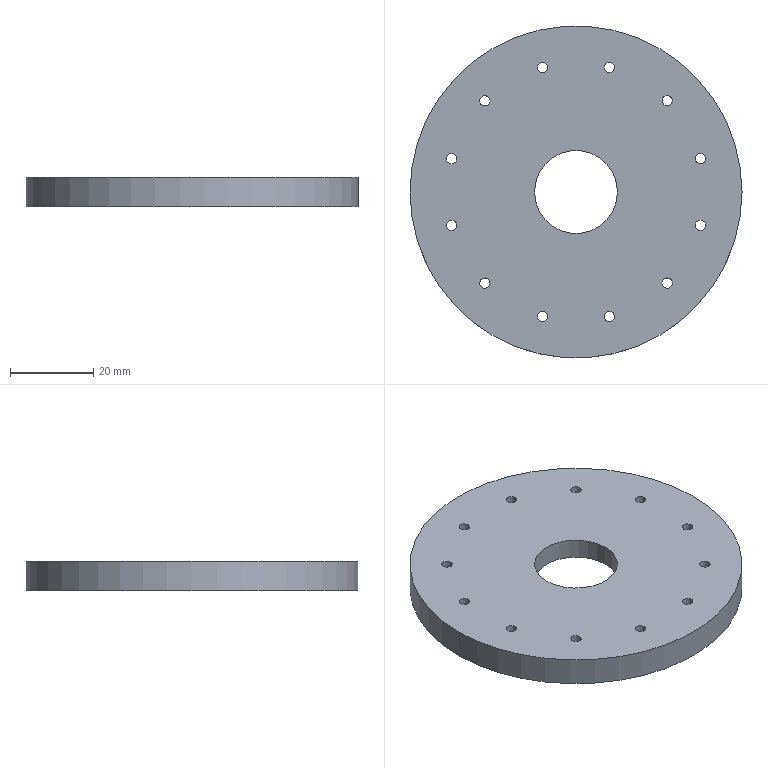Part | NX | features DATUM_CSYS 7, EXTRUDE 7, SKETCH 6, REPLACE_FACE 1 | 1 solid | 18 faces | box 80 x 80 x 7 mm | volume 31789 mm3 | cylinder 15 | plane 3 | commonest cylinder face diameters 2.5 x12 20 x1 30 x1 80 x1
STEP:
#1=CARTESIAN_POINT('',(10.,0.,7.));
#2=VERTEX_POINT('',#1);
#3=CARTESIAN_POINT('',(0.,0.,7.));
#4=DIRECTION('',(0.,0.,1.));
#5=DIRECTION('',(1.,0.,0.));
#6=AXIS2_PLACEMENT_3D('',#3,#4,#5);
#7=CIRCLE('',#6,10.);
#8=EDGE_CURVE('',#2,#2,#7,.T.);
#9=ORIENTED_EDGE('',*,*,#8,.F.);
#10=EDGE_LOOP('',(#9));
#11=FACE_BOUND('',#10,.T.);
#12=CARTESIAN_POINT('',(-28.761,-8.042,7.));
#13=VERTEX_POINT('',#12);
#14=CARTESIAN_POINT('',(-30.011,-8.042,7.));
#15=DIRECTION('',(0.,0.,1.));
#16=DIRECTION('',(1.,0.,0.));
#17=AXIS2_PLACEMENT_3D('',#14,#15,#16);
#18=CIRCLE('',#17,1.25);
#19=EDGE_CURVE('',#13,#13,#18,.T.);
#20=ORIENTED_EDGE('',*,*,#19,.F.);
#21=EDGE_LOOP('',(#20));
#22=FACE_BOUND('',#21,.T.);
#23=CARTESIAN_POINT('',(40.,0.,7.));
#24=VERTEX_POINT('',#23);
#25=CARTESIAN_POINT('',(0.,0.,7.));
#26=DIRECTION('',(0.,0.,1.));
#27=DIRECTION('',(1.,0.,0.));
#28=AXIS2_PLACEMENT_3D('',#25,#26,#27);
#29=CIRCLE('',#28,40.);
#30=EDGE_CURVE('',#24,#24,#29,.T.);
#31=ORIENTED_EDGE('',*,*,#30,.T.);
#32=EDGE_LOOP('',(#31));
#33=FACE_BOUND('',#32,.T.);
#34=CARTESIAN_POINT('',(31.261,8.042,7.));
#35=VERTEX_POINT('',#34);
#36=CARTESIAN_POINT('',(30.011,8.042,7.));
#37=DIRECTION('',(0.,0.,1.));
#38=DIRECTION('',(1.,0.,0.));
#39=AXIS2_PLACEMENT_3D('',#36,#37,#38);
#40=CIRCLE('',#39,1.25);
#41=EDGE_CURVE('',#35,#35,#40,.T.);
#42=ORIENTED_EDGE('',*,*,#41,.F.);
#43=EDGE_LOOP('',(#42));
#44=FACE_BOUND('',#43,.T.);
#45=CARTESIAN_POINT('',(31.261,-8.042,7.));
#46=VERTEX_POINT('',#45);
#47=CARTESIAN_POINT('',(30.011,-8.042,7.));
#48=DIRECTION('',(0.,0.,1.));
#49=DIRECTION('',(1.,0.,0.));
#50=AXIS2_PLACEMENT_3D('',#47,#48,#49);
#51=CIRCLE('',#50,1.25);
#52=EDGE_CURVE('',#46,#46,#51,.T.);
#53=ORIENTED_EDGE('',*,*,#52,.F.);
#54=EDGE_LOOP('',(#53));
#55=FACE_BOUND('',#54,.T.);
#56=CARTESIAN_POINT('',(23.22,21.97,7.));
#57=VERTEX_POINT('',#56);
#58=CARTESIAN_POINT('',(21.97,21.97,7.));
#59=DIRECTION('',(0.,0.,1.));
#60=DIRECTION('',(1.,0.,0.));
#61=AXIS2_PLACEMENT_3D('',#58,#59,#60);
#62=CIRCLE('',#61,1.25);
#63=EDGE_CURVE('',#57,#57,#62,.T.);
#64=ORIENTED_EDGE('',*,*,#63,.F.);
#65=EDGE_LOOP('',(#64));
#66=FACE_BOUND('',#65,.T.);
#67=CARTESIAN_POINT('',(9.292,30.011,7.));
#68=VERTEX_POINT('',#67);
#69=CARTESIAN_POINT('',(8.042,30.011,7.));
#70=DIRECTION('',(0.,0.,1.));
#71=DIRECTION('',(1.,0.,0.));
#72=AXIS2_PLACEMENT_3D('',#69,#70,#71);
#73=CIRCLE('',#72,1.25);
#74=EDGE_CURVE('',#68,#68,#73,.T.);
#75=ORIENTED_EDGE('',*,*,#74,.F.);
#76=EDGE_LOOP('',(#75));
#77=FACE_BOUND('',#76,.T.);
#78=CARTESIAN_POINT('',(23.22,-21.97,7.));
#79=VERTEX_POINT('',#78);
#80=CARTESIAN_POINT('',(21.97,-21.97,7.));
#81=DIRECTION('',(0.,0.,1.));
#82=DIRECTION('',(1.,0.,0.));
#83=AXIS2_PLACEMENT_3D('',#80,#81,#82);
#84=CIRCLE('',#83,1.25);
#85=EDGE_CURVE('',#79,#79,#84,.T.);
#86=ORIENTED_EDGE('',*,*,#85,.F.);
#87=EDGE_LOOP('',(#86));
#88=FACE_BOUND('',#87,.T.);
#89=CARTESIAN_POINT('',(9.292,-30.011,7.));
#90=VERTEX_POINT('',#89);
#91=CARTESIAN_POINT('',(8.042,-30.011,7.));
#92=DIRECTION('',(0.,0.,1.));
#93=DIRECTION('',(1.,0.,0.));
#94=AXIS2_PLACEMENT_3D('',#91,#92,#93);
#95=CIRCLE('',#94,1.25);
#96=EDGE_CURVE('',#90,#90,#95,.T.);
#97=ORIENTED_EDGE('',*,*,#96,.F.);
#98=EDGE_LOOP('',(#97));
#99=FACE_BOUND('',#98,.T.);
#100=CARTESIAN_POINT('',(-6.792,30.011,7.));
#101=VERTEX_POINT('',#100);
#102=CARTESIAN_POINT('',(-8.042,30.011,7.));
#103=DIRECTION('',(0.,0.,1.));
#104=DIRECTION('',(1.,0.,0.));
#105=AXIS2_PLACEMENT_3D('',#102,#103,#104);
#106=CIRCLE('',#105,1.25);
#107=EDGE_CURVE('',#101,#101,#106,.T.);
#108=ORIENTED_EDGE('',*,*,#107,.F.);
#109=EDGE_LOOP('',(#108));
#110=FACE_BOUND('',#109,.T.);
#111=CARTESIAN_POINT('',(-28.761,8.042,7.));
#112=VERTEX_POINT('',#111);
#113=CARTESIAN_POINT('',(-30.011,8.042,7.));
#114=DIRECTION('',(0.,0.,1.));
#115=DIRECTION('',(1.,0.,0.));
#116=AXIS2_PLACEMENT_3D('',#113,#114,#115);
#117=CIRCLE('',#116,1.25);
#118=EDGE_CURVE('',#112,#112,#117,.T.);
#119=ORIENTED_EDGE('',*,*,#118,.F.);
#120=EDGE_LOOP('',(#119));
#121=FACE_BOUND('',#120,.T.);
#122=CARTESIAN_POINT('',(-6.792,-30.011,7.));
#123=VERTEX_POINT('',#122);
#124=CARTESIAN_POINT('',(-8.042,-30.011,7.));
#125=DIRECTION('',(0.,0.,1.));
#126=DIRECTION('',(1.,0.,0.));
#127=AXIS2_PLACEMENT_3D('',#124,#125,#126);
#128=CIRCLE('',#127,1.25);
#129=EDGE_CURVE('',#123,#123,#128,.T.);
#130=ORIENTED_EDGE('',*,*,#129,.F.);
#131=EDGE_LOOP('',(#130));
#132=FACE_BOUND('',#131,.T.);
#133=CARTESIAN_POINT('',(-20.72,21.97,7.));
#134=VERTEX_POINT('',#133);
#135=CARTESIAN_POINT('',(-21.97,21.97,7.));
#136=DIRECTION('',(0.,0.,1.));
#137=DIRECTION('',(1.,0.,0.));
#138=AXIS2_PLACEMENT_3D('',#135,#136,#137);
#139=CIRCLE('',#138,1.25);
#140=EDGE_CURVE('',#134,#134,#139,.T.);
#141=ORIENTED_EDGE('',*,*,#140,.F.);
#142=EDGE_LOOP('',(#141));
#143=FACE_BOUND('',#142,.T.);
#144=CARTESIAN_POINT('',(-20.72,-21.97,7.));
#145=VERTEX_POINT('',#144);
#146=CARTESIAN_POINT('',(-21.97,-21.97,7.));
#147=DIRECTION('',(0.,0.,1.));
#148=DIRECTION('',(1.,0.,0.));
#149=AXIS2_PLACEMENT_3D('',#146,#147,#148);
#150=CIRCLE('',#149,1.25);
#151=EDGE_CURVE('',#145,#145,#150,.T.);
#152=ORIENTED_EDGE('',*,*,#151,.F.);
#153=EDGE_LOOP('',(#152));
#154=FACE_BOUND('',#153,.T.);
#155=CARTESIAN_POINT('',(0.,0.,7.));
#156=DIRECTION('',(0.,0.,1.));
#157=DIRECTION('',(1.,0.,0.));
#158=AXIS2_PLACEMENT_3D('',#155,#156,#157);
#159=PLANE('',#158);
#160=ADVANCED_FACE('',(#11,#22,#33,#44,#55,#66,#77,#88,#99,#110,#121,#132,#143,#154),#159,.T.);
#161=CARTESIAN_POINT('',(40.,0.,0.));
#162=VERTEX_POINT('',#161);
#163=CARTESIAN_POINT('',(0.,0.,0.));
#164=DIRECTION('',(0.,0.,1.));
#165=DIRECTION('',(1.,0.,0.));
#166=AXIS2_PLACEMENT_3D('',#163,#164,#165);
#167=CIRCLE('',#166,40.);
#168=EDGE_CURVE('',#162,#162,#167,.T.);
#169=ORIENTED_EDGE('',*,*,#168,.T.);
#170=EDGE_LOOP('',(#169));
#171=FACE_BOUND('',#170,.T.);
#172=ORIENTED_EDGE('',*,*,#30,.F.);
#173=EDGE_LOOP('',(#172));
#174=FACE_BOUND('',#173,.T.);
#175=CARTESIAN_POINT('',(0.,0.,2.));
#176=DIRECTION('',(0.,0.,-1.));
#177=DIRECTION('',(-1.,0.,0.));
#178=AXIS2_PLACEMENT_3D('',#175,#176,#177);
#179=CYLINDRICAL_SURFACE('',#178,40.);
#180=ADVANCED_FACE('',(#171,#174),#179,.T.);
#181=CARTESIAN_POINT('',(15.,0.,0.));
#182=VERTEX_POINT('',#181);
#183=CARTESIAN_POINT('',(0.,0.,0.));
#184=DIRECTION('',(0.,0.,-1.));
#185=DIRECTION('',(1.,0.,0.));
#186=AXIS2_PLACEMENT_3D('',#183,#184,#185);
#187=CIRCLE('',#186,15.);
#188=EDGE_CURVE('',#182,#182,#187,.T.);
#189=ORIENTED_EDGE('',*,*,#188,.F.);
#190=EDGE_LOOP('',(#189));
#191=FACE_BOUND('',#190,.T.);
#192=CARTESIAN_POINT('',(-8.042,-31.261,0.));
#193=VERTEX_POINT('',#192);
#194=CARTESIAN_POINT('',(-8.042,-30.011,0.));
#195=DIRECTION('',(0.,0.,-1.));
#196=DIRECTION('',(0.,-1.,0.));
#197=AXIS2_PLACEMENT_3D('',#194,#195,#196);
#198=CIRCLE('',#197,1.25);
#199=EDGE_CURVE('',#193,#193,#198,.T.);
#200=ORIENTED_EDGE('',*,*,#199,.F.);
#201=EDGE_LOOP('',(#200));
#202=FACE_BOUND('',#201,.T.);
#203=CARTESIAN_POINT('',(-23.052,22.595,0.));
#204=VERTEX_POINT('',#203);
#205=CARTESIAN_POINT('',(-21.97,21.97,0.));
#206=DIRECTION('',(0.,0.,-1.));
#207=DIRECTION('',(-0.866,0.5,0.));
#208=AXIS2_PLACEMENT_3D('',#205,#206,#207);
#209=CIRCLE('',#208,1.25);
#210=EDGE_CURVE('',#204,#204,#209,.T.);
#211=ORIENTED_EDGE('',*,*,#210,.F.);
#212=EDGE_LOOP('',(#211));
#213=FACE_BOUND('',#212,.T.);
#214=CARTESIAN_POINT('',(-31.261,8.042,0.));
#215=VERTEX_POINT('',#214);
#216=CARTESIAN_POINT('',(-30.011,8.042,0.));
#217=DIRECTION('',(0.,0.,-1.));
#218=DIRECTION('',(-1.,0.,0.));
#219=AXIS2_PLACEMENT_3D('',#216,#217,#218);
#220=CIRCLE('',#219,1.25);
#221=EDGE_CURVE('',#215,#215,#220,.T.);
#222=ORIENTED_EDGE('',*,*,#221,.F.);
#223=EDGE_LOOP('',(#222));
#224=FACE_BOUND('',#223,.T.);
#225=CARTESIAN_POINT('',(-31.094,-8.667,0.));
#226=VERTEX_POINT('',#225);
#227=CARTESIAN_POINT('',(-30.011,-8.042,0.));
#228=DIRECTION('',(0.,0.,-1.));
#229=DIRECTION('',(-0.866,-0.5,0.));
#230=AXIS2_PLACEMENT_3D('',#227,#228,#229);
#231=CIRCLE('',#230,1.25);
#232=EDGE_CURVE('',#226,#226,#231,.T.);
#233=ORIENTED_EDGE('',*,*,#232,.F.);
#234=EDGE_LOOP('',(#233));
#235=FACE_BOUND('',#234,.T.);
#236=CARTESIAN_POINT('',(-22.595,-23.052,0.));
#237=VERTEX_POINT('',#236);
#238=CARTESIAN_POINT('',(-21.97,-21.97,0.));
#239=DIRECTION('',(0.,0.,-1.));
#240=DIRECTION('',(-0.5,-0.866,0.));
#241=AXIS2_PLACEMENT_3D('',#238,#239,#240);
#242=CIRCLE('',#241,1.25);
#243=EDGE_CURVE('',#237,#237,#242,.T.);
#244=ORIENTED_EDGE('',*,*,#243,.F.);
#245=EDGE_LOOP('',(#244));
#246=FACE_BOUND('',#245,.T.);
#247=CARTESIAN_POINT('',(-8.667,31.094,0.));
#248=VERTEX_POINT('',#247);
#249=CARTESIAN_POINT('',(-8.042,30.011,0.));
#250=DIRECTION('',(0.,0.,-1.));
#251=DIRECTION('',(-0.5,0.866,0.));
#252=AXIS2_PLACEMENT_3D('',#249,#250,#251);
#253=CIRCLE('',#252,1.25);
#254=EDGE_CURVE('',#248,#248,#253,.T.);
#255=ORIENTED_EDGE('',*,*,#254,.F.);
#256=EDGE_LOOP('',(#255));
#257=FACE_BOUND('',#256,.T.);
#258=CARTESIAN_POINT('',(8.667,-31.094,0.));
#259=VERTEX_POINT('',#258);
#260=CARTESIAN_POINT('',(8.042,-30.011,0.));
#261=DIRECTION('',(0.,0.,-1.));
#262=DIRECTION('',(0.5,-0.866,0.));
#263=AXIS2_PLACEMENT_3D('',#260,#261,#262);
#264=CIRCLE('',#263,1.25);
#265=EDGE_CURVE('',#259,#259,#264,.T.);
#266=ORIENTED_EDGE('',*,*,#265,.F.);
#267=EDGE_LOOP('',(#266));
#268=FACE_BOUND('',#267,.T.);
#269=CARTESIAN_POINT('',(23.052,-22.595,0.));
#270=VERTEX_POINT('',#269);
#271=CARTESIAN_POINT('',(21.97,-21.97,0.));
#272=DIRECTION('',(0.,0.,-1.));
#273=DIRECTION('',(0.866,-0.5,0.));
#274=AXIS2_PLACEMENT_3D('',#271,#272,#273);
#275=CIRCLE('',#274,1.25);
#276=EDGE_CURVE('',#270,#270,#275,.T.);
#277=ORIENTED_EDGE('',*,*,#276,.F.);
#278=EDGE_LOOP('',(#277));
#279=FACE_BOUND('',#278,.T.);
#280=CARTESIAN_POINT('',(8.042,31.261,0.));
#281=VERTEX_POINT('',#280);
#282=CARTESIAN_POINT('',(8.042,30.011,0.));
#283=DIRECTION('',(0.,0.,-1.));
#284=DIRECTION('',(0.,1.,0.));
#285=AXIS2_PLACEMENT_3D('',#282,#283,#284);
#286=CIRCLE('',#285,1.25);
#287=EDGE_CURVE('',#281,#281,#286,.T.);
#288=ORIENTED_EDGE('',*,*,#287,.F.);
#289=EDGE_LOOP('',(#288));
#290=FACE_BOUND('',#289,.T.);
#291=CARTESIAN_POINT('',(22.595,23.052,0.));
#292=VERTEX_POINT('',#291);
#293=CARTESIAN_POINT('',(21.97,21.97,0.));
#294=DIRECTION('',(0.,0.,-1.));
#295=DIRECTION('',(0.5,0.866,0.));
#296=AXIS2_PLACEMENT_3D('',#293,#294,#295);
#297=CIRCLE('',#296,1.25);
#298=EDGE_CURVE('',#292,#292,#297,.T.);
#299=ORIENTED_EDGE('',*,*,#298,.F.);
#300=EDGE_LOOP('',(#299));
#301=FACE_BOUND('',#300,.T.);
#302=CARTESIAN_POINT('',(31.261,-8.042,0.));
#303=VERTEX_POINT('',#302);
#304=CARTESIAN_POINT('',(30.011,-8.042,0.));
#305=DIRECTION('',(0.,0.,-1.));
#306=DIRECTION('',(1.,0.,0.));
#307=AXIS2_PLACEMENT_3D('',#304,#305,#306);
#308=CIRCLE('',#307,1.25);
#309=EDGE_CURVE('',#303,#303,#308,.T.);
#310=ORIENTED_EDGE('',*,*,#309,.F.);
#311=EDGE_LOOP('',(#310));
#312=FACE_BOUND('',#311,.T.);
#313=CARTESIAN_POINT('',(31.094,8.667,0.));
#314=VERTEX_POINT('',#313);
#315=CARTESIAN_POINT('',(30.011,8.042,0.));
#316=DIRECTION('',(0.,0.,-1.));
#317=DIRECTION('',(0.866,0.5,0.));
#318=AXIS2_PLACEMENT_3D('',#315,#316,#317);
#319=CIRCLE('',#318,1.25);
#320=EDGE_CURVE('',#314,#314,#319,.T.);
#321=ORIENTED_EDGE('',*,*,#320,.F.);
#322=EDGE_LOOP('',(#321));
#323=FACE_BOUND('',#322,.T.);
#324=ORIENTED_EDGE('',*,*,#168,.F.);
#325=EDGE_LOOP('',(#324));
#326=FACE_BOUND('',#325,.T.);
#327=CARTESIAN_POINT('',(0.,0.,0.));
#328=DIRECTION('',(0.,0.,1.));
#329=DIRECTION('',(1.,0.,0.));
#330=AXIS2_PLACEMENT_3D('',#327,#328,#329);
#331=PLANE('',#330);
#332=ADVANCED_FACE('',(#191,#202,#213,#224,#235,#246,#257,#268,#279,#290,#301,#312,#323,#326),#331,.F.);
#333=ORIENTED_EDGE('',*,*,#320,.T.);
#334=EDGE_LOOP('',(#333));
#335=FACE_BOUND('',#334,.T.);
#336=ORIENTED_EDGE('',*,*,#41,.T.);
#337=EDGE_LOOP('',(#336));
#338=FACE_BOUND('',#337,.T.);
#339=CARTESIAN_POINT('',(30.011,8.042,39.));
#340=DIRECTION('',(0.,0.,-1.));
#341=DIRECTION('',(-1.,0.,0.));
#342=AXIS2_PLACEMENT_3D('',#339,#340,#341);
#343=CYLINDRICAL_SURFACE('',#342,1.25);
#344=ADVANCED_FACE('',(#335,#338),#343,.F.);
#345=ORIENTED_EDGE('',*,*,#309,.T.);
#346=EDGE_LOOP('',(#345));
#347=FACE_BOUND('',#346,.T.);
#348=ORIENTED_EDGE('',*,*,#52,.T.);
#349=EDGE_LOOP('',(#348));
#350=FACE_BOUND('',#349,.T.);
#351=CARTESIAN_POINT('',(30.011,-8.042,39.));
#352=DIRECTION('',(0.,0.,-1.));
#353=DIRECTION('',(-1.,0.,0.));
#354=AXIS2_PLACEMENT_3D('',#351,#352,#353);
#355=CYLINDRICAL_SURFACE('',#354,1.25);
#356=ADVANCED_FACE('',(#347,#350),#355,.F.);
#357=ORIENTED_EDGE('',*,*,#298,.T.);
#358=EDGE_LOOP('',(#357));
#359=FACE_BOUND('',#358,.T.);
#360=ORIENTED_EDGE('',*,*,#63,.T.);
#361=EDGE_LOOP('',(#360));
#362=FACE_BOUND('',#361,.T.);
#363=CARTESIAN_POINT('',(21.97,21.97,39.));
#364=DIRECTION('',(0.,0.,-1.));
#365=DIRECTION('',(-1.,0.,0.));
#366=AXIS2_PLACEMENT_3D('',#363,#364,#365);
#367=CYLINDRICAL_SURFACE('',#366,1.25);
#368=ADVANCED_FACE('',(#359,#362),#367,.F.);
#369=ORIENTED_EDGE('',*,*,#287,.T.);
#370=EDGE_LOOP('',(#369));
#371=FACE_BOUND('',#370,.T.);
#372=ORIENTED_EDGE('',*,*,#74,.T.);
#373=EDGE_LOOP('',(#372));
#374=FACE_BOUND('',#373,.T.);
#375=CARTESIAN_POINT('',(8.042,30.011,39.));
#376=DIRECTION('',(0.,0.,-1.));
#377=DIRECTION('',(-1.,0.,0.));
#378=AXIS2_PLACEMENT_3D('',#375,#376,#377);
#379=CYLINDRICAL_SURFACE('',#378,1.25);
#380=ADVANCED_FACE('',(#371,#374),#379,.F.);
#381=ORIENTED_EDGE('',*,*,#276,.T.);
#382=EDGE_LOOP('',(#381));
#383=FACE_BOUND('',#382,.T.);
#384=ORIENTED_EDGE('',*,*,#85,.T.);
#385=EDGE_LOOP('',(#384));
#386=FACE_BOUND('',#385,.T.);
#387=CARTESIAN_POINT('',(21.97,-21.97,39.));
#388=DIRECTION('',(0.,0.,-1.));
#389=DIRECTION('',(-1.,0.,0.));
#390=AXIS2_PLACEMENT_3D('',#387,#388,#389);
#391=CYLINDRICAL_SURFACE('',#390,1.25);
#392=ADVANCED_FACE('',(#383,#386),#391,.F.);
#393=ORIENTED_EDGE('',*,*,#265,.T.);
#394=EDGE_LOOP('',(#393));
#395=FACE_BOUND('',#394,.T.);
#396=ORIENTED_EDGE('',*,*,#96,.T.);
#397=EDGE_LOOP('',(#396));
#398=FACE_BOUND('',#397,.T.);
#399=CARTESIAN_POINT('',(8.042,-30.011,39.));
#400=DIRECTION('',(0.,0.,-1.));
#401=DIRECTION('',(-1.,0.,0.));
#402=AXIS2_PLACEMENT_3D('',#399,#400,#401);
#403=CYLINDRICAL_SURFACE('',#402,1.25);
#404=ADVANCED_FACE('',(#395,#398),#403,.F.);
#405=ORIENTED_EDGE('',*,*,#254,.T.);
#406=EDGE_LOOP('',(#405));
#407=FACE_BOUND('',#406,.T.);
#408=ORIENTED_EDGE('',*,*,#107,.T.);
#409=EDGE_LOOP('',(#408));
#410=FACE_BOUND('',#409,.T.);
#411=CARTESIAN_POINT('',(-8.042,30.011,39.));
#412=DIRECTION('',(0.,0.,-1.));
#413=DIRECTION('',(-1.,0.,0.));
#414=AXIS2_PLACEMENT_3D('',#411,#412,#413);
#415=CYLINDRICAL_SURFACE('',#414,1.25);
#416=ADVANCED_FACE('',(#407,#410),#415,.F.);
#417=ORIENTED_EDGE('',*,*,#243,.T.);
#418=EDGE_LOOP('',(#417));
#419=FACE_BOUND('',#418,.T.);
#420=ORIENTED_EDGE('',*,*,#151,.T.);
#421=EDGE_LOOP('',(#420));
#422=FACE_BOUND('',#421,.T.);
#423=CARTESIAN_POINT('',(-21.97,-21.97,39.));
#424=DIRECTION('',(0.,0.,-1.));
#425=DIRECTION('',(-1.,0.,0.));
#426=AXIS2_PLACEMENT_3D('',#423,#424,#425);
#427=CYLINDRICAL_SURFACE('',#426,1.25);
#428=ADVANCED_FACE('',(#419,#422),#427,.F.);
#429=ORIENTED_EDGE('',*,*,#232,.T.);
#430=EDGE_LOOP('',(#429));
#431=FACE_BOUND('',#430,.T.);
#432=ORIENTED_EDGE('',*,*,#19,.T.);
#433=EDGE_LOOP('',(#432));
#434=FACE_BOUND('',#433,.T.);
#435=CARTESIAN_POINT('',(-30.011,-8.042,39.));
#436=DIRECTION('',(0.,0.,-1.));
#437=DIRECTION('',(-1.,0.,0.));
#438=AXIS2_PLACEMENT_3D('',#435,#436,#437);
#439=CYLINDRICAL_SURFACE('',#438,1.25);
#440=ADVANCED_FACE('',(#431,#434),#439,.F.);
#441=ORIENTED_EDGE('',*,*,#221,.T.);
#442=EDGE_LOOP('',(#441));
#443=FACE_BOUND('',#442,.T.);
#444=ORIENTED_EDGE('',*,*,#118,.T.);
#445=EDGE_LOOP('',(#444));
#446=FACE_BOUND('',#445,.T.);
#447=CARTESIAN_POINT('',(-30.011,8.042,39.));
#448=DIRECTION('',(0.,0.,-1.));
#449=DIRECTION('',(-1.,0.,0.));
#450=AXIS2_PLACEMENT_3D('',#447,#448,#449);
#451=CYLINDRICAL_SURFACE('',#450,1.25);
#452=ADVANCED_FACE('',(#443,#446),#451,.F.);
#453=ORIENTED_EDGE('',*,*,#210,.T.);
#454=EDGE_LOOP('',(#453));
#455=FACE_BOUND('',#454,.T.);
#456=ORIENTED_EDGE('',*,*,#140,.T.);
#457=EDGE_LOOP('',(#456));
#458=FACE_BOUND('',#457,.T.);
#459=CARTESIAN_POINT('',(-21.97,21.97,39.));
#460=DIRECTION('',(0.,0.,-1.));
#461=DIRECTION('',(-1.,0.,0.));
#462=AXIS2_PLACEMENT_3D('',#459,#460,#461);
#463=CYLINDRICAL_SURFACE('',#462,1.25);
#464=ADVANCED_FACE('',(#455,#458),#463,.F.);
#465=ORIENTED_EDGE('',*,*,#199,.T.);
#466=EDGE_LOOP('',(#465));
#467=FACE_BOUND('',#466,.T.);
#468=ORIENTED_EDGE('',*,*,#129,.T.);
#469=EDGE_LOOP('',(#468));
#470=FACE_BOUND('',#469,.T.);
#471=CARTESIAN_POINT('',(-8.042,-30.011,39.));
#472=DIRECTION('',(0.,0.,-1.));
#473=DIRECTION('',(-1.,0.,0.));
#474=AXIS2_PLACEMENT_3D('',#471,#472,#473);
#475=CYLINDRICAL_SURFACE('',#474,1.25);
#476=ADVANCED_FACE('',(#467,#470),#475,.F.);
#477=CARTESIAN_POINT('',(-10.,0.,2.));
#478=VERTEX_POINT('',#477);
#479=CARTESIAN_POINT('',(0.,0.,2.));
#480=DIRECTION('',(0.,0.,-1.));
#481=DIRECTION('',(-1.,0.,0.));
#482=AXIS2_PLACEMENT_3D('',#479,#480,#481);
#483=CIRCLE('',#482,10.);
#484=EDGE_CURVE('',#478,#478,#483,.T.);
#485=ORIENTED_EDGE('',*,*,#484,.F.);
#486=EDGE_LOOP('',(#485));
#487=FACE_BOUND('',#486,.T.);
#488=CARTESIAN_POINT('',(15.,0.,2.));
#489=VERTEX_POINT('',#488);
#490=CARTESIAN_POINT('',(0.,0.,2.));
#491=DIRECTION('',(0.,0.,-1.));
#492=DIRECTION('',(1.,0.,0.));
#493=AXIS2_PLACEMENT_3D('',#490,#491,#492);
#494=CIRCLE('',#493,15.);
#495=EDGE_CURVE('',#489,#489,#494,.F.);
#496=ORIENTED_EDGE('',*,*,#495,.F.);
#497=EDGE_LOOP('',(#496));
#498=FACE_BOUND('',#497,.T.);
#499=CARTESIAN_POINT('',(0.,0.,2.));
#500=DIRECTION('',(0.,0.,-1.));
#501=DIRECTION('',(-1.,0.,0.));
#502=AXIS2_PLACEMENT_3D('',#499,#500,#501);
#503=PLANE('',#502);
#504=ADVANCED_FACE('',(#487,#498),#503,.T.);
#505=ORIENTED_EDGE('',*,*,#495,.T.);
#506=EDGE_LOOP('',(#505));
#507=FACE_BOUND('',#506,.T.);
#508=ORIENTED_EDGE('',*,*,#188,.T.);
#509=EDGE_LOOP('',(#508));
#510=FACE_BOUND('',#509,.T.);
#511=CARTESIAN_POINT('',(0.,0.,2.));
#512=DIRECTION('',(0.,0.,-1.));
#513=DIRECTION('',(-1.,0.,0.));
#514=AXIS2_PLACEMENT_3D('',#511,#512,#513);
#515=CYLINDRICAL_SURFACE('',#514,15.);
#516=ADVANCED_FACE('',(#507,#510),#515,.F.);
#517=ORIENTED_EDGE('',*,*,#484,.T.);
#518=EDGE_LOOP('',(#517));
#519=FACE_BOUND('',#518,.T.);
#520=ORIENTED_EDGE('',*,*,#8,.T.);
#521=EDGE_LOOP('',(#520));
#522=FACE_BOUND('',#521,.T.);
#523=CARTESIAN_POINT('',(0.,0.,-23.));
#524=DIRECTION('',(0.,0.,1.));
#525=DIRECTION('',(1.,0.,0.));
#526=AXIS2_PLACEMENT_3D('',#523,#524,#525);
#527=CYLINDRICAL_SURFACE('',#526,10.);
#528=ADVANCED_FACE('',(#519,#522),#527,.F.);
#529=CLOSED_SHELL('',(#160,#180,#332,#344,#356,#368,#380,#392,#404,#416,#428,#440,#452,#464,#476,#504,#516,#528));
#530=MANIFOLD_SOLID_BREP('',#529);
#531=(LENGTH_UNIT()NAMED_UNIT(*)SI_UNIT(.MILLI.,.METRE.));
#532=UNCERTAINTY_MEASURE_WITH_UNIT(LENGTH_MEASURE(0.00001),#531,'','');
#533=(NAMED_UNIT(*)PLANE_ANGLE_UNIT()SI_UNIT($,.RADIAN.));
#534=(NAMED_UNIT(*)SI_UNIT($,.STERADIAN.)SOLID_ANGLE_UNIT());
#535=(GEOMETRIC_REPRESENTATION_CONTEXT(3)GLOBAL_UNCERTAINTY_ASSIGNED_CONTEXT((#532))GLOBAL_UNIT_ASSIGNED_CONTEXT((#531,#533,#534))REPRESENTATION_CONTEXT('',''));
#536=ADVANCED_BREP_SHAPE_REPRESENTATION('',(#530),#535);